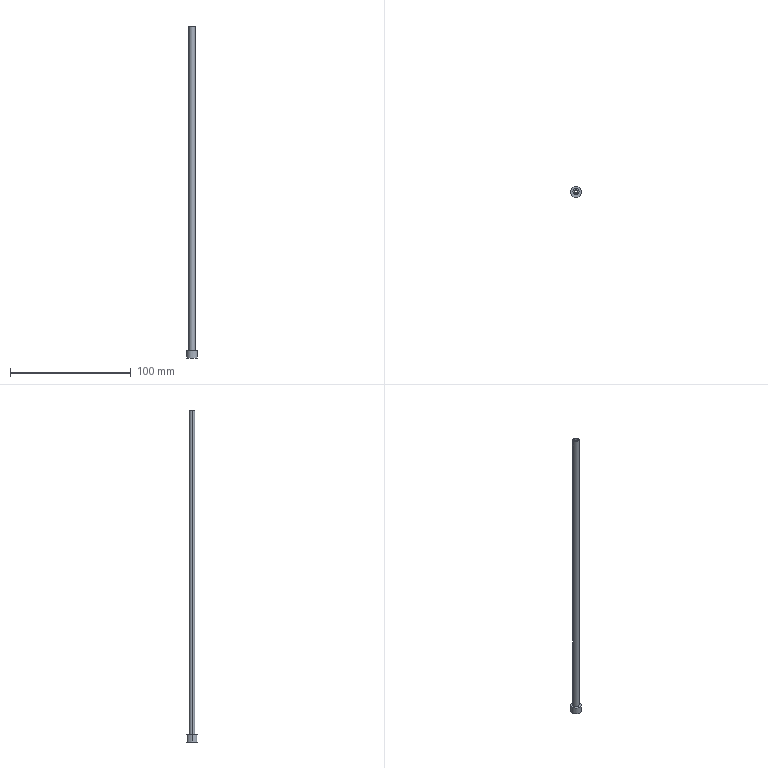Part | Creo | 1 solid | 12 faces | box 9 x 9 x 275.272 mm | volume 3782 mm3 | cylinder 8 | plane 4 | commonest cylinder face diameters 2.8 x2 3 x2 5 x2 9 x2
STEP:
#1=CARTESIAN_POINT('',(52.238,-56.28,-296.));
#2=VERTEX_POINT('',#1);
#3=CARTESIAN_POINT('',(43.238,-56.28,-296.));
#4=VERTEX_POINT('',#3);
#5=CARTESIAN_POINT('',(47.738,-56.28,-296.));
#6=DIRECTION('',(0.,0.,-1.));
#7=DIRECTION('',(1.,0.,0.));
#8=AXIS2_PLACEMENT_3D('',#5,#6,#7);
#9=CIRCLE('',#8,4.5);
#10=EDGE_CURVE('',#2,#4,#9,.T.);
#11=ORIENTED_EDGE('',*,*,#10,.F.);
#12=CARTESIAN_POINT('',(47.738,-56.28,-296.));
#13=DIRECTION('',(0.,0.,-1.));
#14=DIRECTION('',(-1.,0.,0.));
#15=AXIS2_PLACEMENT_3D('',#12,#13,#14);
#16=CIRCLE('',#15,4.5);
#17=EDGE_CURVE('',#4,#2,#16,.T.);
#18=ORIENTED_EDGE('',*,*,#17,.F.);
#19=EDGE_LOOP('',(#11,#18));
#20=FACE_OUTER_BOUND('',#19,.F.);
#21=CARTESIAN_POINT('',(49.238,-56.28,-296.));
#22=VERTEX_POINT('',#21);
#23=CARTESIAN_POINT('',(46.238,-56.28,-296.));
#24=VERTEX_POINT('',#23);
#25=CARTESIAN_POINT('',(47.738,-56.28,-296.));
#26=DIRECTION('',(0.,0.,1.));
#27=DIRECTION('',(1.,0.,0.));
#28=AXIS2_PLACEMENT_3D('',#25,#26,#27);
#29=CIRCLE('',#28,1.5);
#30=EDGE_CURVE('',#22,#24,#29,.T.);
#31=ORIENTED_EDGE('',*,*,#30,.F.);
#32=CARTESIAN_POINT('',(47.738,-56.28,-296.));
#33=DIRECTION('',(0.,0.,1.));
#34=DIRECTION('',(-1.,0.,0.));
#35=AXIS2_PLACEMENT_3D('',#32,#33,#34);
#36=CIRCLE('',#35,1.5);
#37=EDGE_CURVE('',#24,#22,#36,.T.);
#38=ORIENTED_EDGE('',*,*,#37,.F.);
#39=EDGE_LOOP('',(#31,#38));
#40=FACE_BOUND('',#39,.F.);
#41=CARTESIAN_POINT('',(10.,-0.004699,-296.));
#42=DIRECTION('',(0.,0.,1.));
#43=DIRECTION('',(0.,1.,0.));
#44=AXIS2_PLACEMENT_3D('',#41,#42,#43);
#45=PLANE('',#44);
#46=ADVANCED_FACE('',(#20,#40),#45,.F.);
#47=CARTESIAN_POINT('',(43.238,-56.28,-290.));
#48=VERTEX_POINT('',#47);
#49=CARTESIAN_POINT('',(52.238,-56.28,-290.));
#50=VERTEX_POINT('',#49);
#51=CARTESIAN_POINT('',(47.738,-56.28,-290.));
#52=DIRECTION('',(0.,0.,1.));
#53=DIRECTION('',(-1.,0.,0.));
#54=AXIS2_PLACEMENT_3D('',#51,#52,#53);
#55=CIRCLE('',#54,4.5);
#56=EDGE_CURVE('',#48,#50,#55,.T.);
#57=ORIENTED_EDGE('',*,*,#56,.T.);
#58=CARTESIAN_POINT('',(52.238,-56.28,-296.));
#59=DIRECTION('',(0.,0.,1.));
#60=VECTOR('',#59,6.);
#61=LINE('',#58,#60);
#62=EDGE_CURVE('',#2,#50,#61,.T.);
#63=ORIENTED_EDGE('',*,*,#62,.F.);
#64=ORIENTED_EDGE('',*,*,#10,.T.);
#65=CARTESIAN_POINT('',(43.238,-56.28,-296.));
#66=DIRECTION('',(0.,0.,1.));
#67=VECTOR('',#66,6.);
#68=LINE('',#65,#67);
#69=EDGE_CURVE('',#4,#48,#68,.T.);
#70=ORIENTED_EDGE('',*,*,#69,.T.);
#71=EDGE_LOOP('',(#57,#63,#64,#70));
#72=FACE_OUTER_BOUND('',#71,.F.);
#73=CARTESIAN_POINT('',(47.738,-56.28,-296.));
#74=DIRECTION('',(0.,0.,1.));
#75=DIRECTION('',(-1.,0.,0.));
#76=AXIS2_PLACEMENT_3D('',#73,#74,#75);
#77=CYLINDRICAL_SURFACE('',#76,4.5);
#78=ADVANCED_FACE('',(#72),#77,.T.);
#79=CARTESIAN_POINT('',(47.738,-56.28,-290.));
#80=DIRECTION('',(0.,0.,1.));
#81=DIRECTION('',(1.,0.,0.));
#82=AXIS2_PLACEMENT_3D('',#79,#80,#81);
#83=CIRCLE('',#82,4.5);
#84=EDGE_CURVE('',#50,#48,#83,.T.);
#85=ORIENTED_EDGE('',*,*,#84,.F.);
#86=ORIENTED_EDGE('',*,*,#56,.F.);
#87=EDGE_LOOP('',(#85,#86));
#88=FACE_OUTER_BOUND('',#87,.F.);
#89=CARTESIAN_POINT('',(50.238,-56.28,-290.));
#90=VERTEX_POINT('',#89);
#91=CARTESIAN_POINT('',(45.238,-56.28,-290.));
#92=VERTEX_POINT('',#91);
#93=CARTESIAN_POINT('',(47.738,-56.28,-290.));
#94=DIRECTION('',(0.,0.,-1.));
#95=DIRECTION('',(1.,0.,0.));
#96=AXIS2_PLACEMENT_3D('',#93,#94,#95);
#97=CIRCLE('',#96,2.5);
#98=EDGE_CURVE('',#90,#92,#97,.T.);
#99=ORIENTED_EDGE('',*,*,#98,.F.);
#100=CARTESIAN_POINT('',(47.738,-56.28,-290.));
#101=DIRECTION('',(0.,0.,-1.));
#102=DIRECTION('',(-1.,0.,0.));
#103=AXIS2_PLACEMENT_3D('',#100,#101,#102);
#104=CIRCLE('',#103,2.5);
#105=EDGE_CURVE('',#92,#90,#104,.T.);
#106=ORIENTED_EDGE('',*,*,#105,.F.);
#107=EDGE_LOOP('',(#99,#106));
#108=FACE_BOUND('',#107,.F.);
#109=CARTESIAN_POINT('',(47.738,-56.28,-290.));
#110=DIRECTION('',(0.,0.,1.));
#111=DIRECTION('',(-1.,0.,0.));
#112=AXIS2_PLACEMENT_3D('',#109,#110,#111);
#113=PLANE('',#112);
#114=ADVANCED_FACE('',(#88,#108),#113,.T.);
#115=ORIENTED_EDGE('',*,*,#98,.T.);
#116=CARTESIAN_POINT('',(45.238,-56.28,-20.728));
#117=VERTEX_POINT('',#116);
#118=CARTESIAN_POINT('',(45.238,-56.28,-290.));
#119=DIRECTION('',(0.,0.,1.));
#120=VECTOR('',#119,269.272);
#121=LINE('',#118,#120);
#122=EDGE_CURVE('',#92,#117,#121,.T.);
#123=ORIENTED_EDGE('',*,*,#122,.T.);
#124=CARTESIAN_POINT('',(50.238,-56.28,-20.728));
#125=VERTEX_POINT('',#124);
#126=CARTESIAN_POINT('',(47.738,-56.28,-20.728));
#127=DIRECTION('',(0.,0.,1.));
#128=DIRECTION('',(-1.,0.,0.));
#129=AXIS2_PLACEMENT_3D('',#126,#127,#128);
#130=CIRCLE('',#129,2.5);
#131=EDGE_CURVE('',#117,#125,#130,.T.);
#132=ORIENTED_EDGE('',*,*,#131,.T.);
#133=CARTESIAN_POINT('',(50.238,-56.28,-290.));
#134=DIRECTION('',(0.,0.,1.));
#135=VECTOR('',#134,269.272);
#136=LINE('',#133,#135);
#137=EDGE_CURVE('',#90,#125,#136,.T.);
#138=ORIENTED_EDGE('',*,*,#137,.F.);
#139=EDGE_LOOP('',(#115,#123,#132,#138));
#140=FACE_OUTER_BOUND('',#139,.F.);
#141=CARTESIAN_POINT('',(47.738,-56.28,-335.923));
#142=DIRECTION('',(0.,0.,1.));
#143=DIRECTION('',(1.,0.,0.));
#144=AXIS2_PLACEMENT_3D('',#141,#142,#143);
#145=CYLINDRICAL_SURFACE('',#144,2.5);
#146=ADVANCED_FACE('',(#140),#145,.T.);
#147=ORIENTED_EDGE('',*,*,#105,.T.);
#148=ORIENTED_EDGE('',*,*,#137,.T.);
#149=CARTESIAN_POINT('',(47.738,-56.28,-20.728));
#150=DIRECTION('',(0.,0.,1.));
#151=DIRECTION('',(1.,0.,0.));
#152=AXIS2_PLACEMENT_3D('',#149,#150,#151);
#153=CIRCLE('',#152,2.5);
#154=EDGE_CURVE('',#125,#117,#153,.T.);
#155=ORIENTED_EDGE('',*,*,#154,.T.);
#156=ORIENTED_EDGE('',*,*,#122,.F.);
#157=EDGE_LOOP('',(#147,#148,#155,#156));
#158=FACE_OUTER_BOUND('',#157,.F.);
#159=CARTESIAN_POINT('',(47.738,-56.28,-335.923));
#160=DIRECTION('',(0.,0.,1.));
#161=DIRECTION('',(1.,0.,0.));
#162=AXIS2_PLACEMENT_3D('',#159,#160,#161);
#163=CYLINDRICAL_SURFACE('',#162,2.5);
#164=ADVANCED_FACE('',(#158),#163,.T.);
#165=ORIENTED_EDGE('',*,*,#154,.F.);
#166=ORIENTED_EDGE('',*,*,#131,.F.);
#167=EDGE_LOOP('',(#165,#166));
#168=FACE_OUTER_BOUND('',#167,.F.);
#169=CARTESIAN_POINT('',(49.138,-56.28,-20.728));
#170=VERTEX_POINT('',#169);
#171=CARTESIAN_POINT('',(46.338,-56.28,-20.728));
#172=VERTEX_POINT('',#171);
#173=CARTESIAN_POINT('',(47.738,-56.28,-20.728));
#174=DIRECTION('',(0.,0.,-1.));
#175=DIRECTION('',(1.,0.,0.));
#176=AXIS2_PLACEMENT_3D('',#173,#174,#175);
#177=CIRCLE('',#176,1.4);
#178=EDGE_CURVE('',#170,#172,#177,.T.);
#179=ORIENTED_EDGE('',*,*,#178,.F.);
#180=CARTESIAN_POINT('',(47.738,-56.28,-20.728));
#181=DIRECTION('',(0.,0.,-1.));
#182=DIRECTION('',(-1.,0.,0.));
#183=AXIS2_PLACEMENT_3D('',#180,#181,#182);
#184=CIRCLE('',#183,1.4);
#185=EDGE_CURVE('',#172,#170,#184,.T.);
#186=ORIENTED_EDGE('',*,*,#185,.F.);
#187=EDGE_LOOP('',(#179,#186));
#188=FACE_BOUND('',#187,.F.);
#189=CARTESIAN_POINT('',(47.738,-56.28,-20.728));
#190=DIRECTION('',(0.,0.,1.));
#191=DIRECTION('',(1.,0.,0.));
#192=AXIS2_PLACEMENT_3D('',#189,#190,#191);
#193=PLANE('',#192);
#194=ADVANCED_FACE('',(#168,#188),#193,.T.);
#195=CARTESIAN_POINT('',(46.338,-56.28,-85.923));
#196=VERTEX_POINT('',#195);
#197=CARTESIAN_POINT('',(49.138,-56.28,-85.923));
#198=VERTEX_POINT('',#197);
#199=CARTESIAN_POINT('',(47.738,-56.28,-85.923));
#200=DIRECTION('',(0.,0.,1.));
#201=DIRECTION('',(-1.,0.,0.));
#202=AXIS2_PLACEMENT_3D('',#199,#200,#201);
#203=CIRCLE('',#202,1.4);
#204=EDGE_CURVE('',#196,#198,#203,.T.);
#205=ORIENTED_EDGE('',*,*,#204,.T.);
#206=CARTESIAN_POINT('',(49.138,-56.28,-85.923));
#207=DIRECTION('',(0.,0.,1.));
#208=VECTOR('',#207,65.195);
#209=LINE('',#206,#208);
#210=EDGE_CURVE('',#198,#170,#209,.T.);
#211=ORIENTED_EDGE('',*,*,#210,.T.);
#212=ORIENTED_EDGE('',*,*,#178,.T.);
#213=CARTESIAN_POINT('',(46.338,-56.28,-85.923));
#214=DIRECTION('',(0.,0.,1.));
#215=VECTOR('',#214,65.195);
#216=LINE('',#213,#215);
#217=EDGE_CURVE('',#196,#172,#216,.T.);
#218=ORIENTED_EDGE('',*,*,#217,.F.);
#219=EDGE_LOOP('',(#205,#211,#212,#218));
#220=FACE_OUTER_BOUND('',#219,.F.);
#221=CARTESIAN_POINT('',(47.738,-56.28,-335.923));
#222=DIRECTION('',(0.,0.,1.));
#223=DIRECTION('',(1.,0.,0.));
#224=AXIS2_PLACEMENT_3D('',#221,#222,#223);
#225=CYLINDRICAL_SURFACE('',#224,1.4);
#226=ADVANCED_FACE('',(#220),#225,.F.);
#227=CARTESIAN_POINT('',(49.238,-56.28,-85.923));
#228=VERTEX_POINT('',#227);
#229=CARTESIAN_POINT('',(46.238,-56.28,-85.923));
#230=VERTEX_POINT('',#229);
#231=CARTESIAN_POINT('',(47.738,-56.28,-85.923));
#232=DIRECTION('',(0.,0.,-1.));
#233=DIRECTION('',(1.,0.,0.));
#234=AXIS2_PLACEMENT_3D('',#231,#232,#233);
#235=CIRCLE('',#234,1.5);
#236=EDGE_CURVE('',#228,#230,#235,.T.);
#237=ORIENTED_EDGE('',*,*,#236,.F.);
#238=CARTESIAN_POINT('',(47.738,-56.28,-85.923));
#239=DIRECTION('',(0.,0.,-1.));
#240=DIRECTION('',(-1.,0.,0.));
#241=AXIS2_PLACEMENT_3D('',#238,#239,#240);
#242=CIRCLE('',#241,1.5);
#243=EDGE_CURVE('',#230,#228,#242,.T.);
#244=ORIENTED_EDGE('',*,*,#243,.F.);
#245=EDGE_LOOP('',(#237,#244));
#246=FACE_OUTER_BOUND('',#245,.F.);
#247=CARTESIAN_POINT('',(47.738,-56.28,-85.923));
#248=DIRECTION('',(0.,0.,1.));
#249=DIRECTION('',(1.,0.,0.));
#250=AXIS2_PLACEMENT_3D('',#247,#248,#249);
#251=CIRCLE('',#250,1.4);
#252=EDGE_CURVE('',#198,#196,#251,.T.);
#253=ORIENTED_EDGE('',*,*,#252,.F.);
#254=ORIENTED_EDGE('',*,*,#204,.F.);
#255=EDGE_LOOP('',(#253,#254));
#256=FACE_BOUND('',#255,.F.);
#257=CARTESIAN_POINT('',(47.738,-56.28,-85.923));
#258=DIRECTION('',(0.,0.,1.));
#259=DIRECTION('',(1.,0.,0.));
#260=AXIS2_PLACEMENT_3D('',#257,#258,#259);
#261=PLANE('',#260);
#262=ADVANCED_FACE('',(#246,#256),#261,.F.);
#263=ORIENTED_EDGE('',*,*,#37,.T.);
#264=CARTESIAN_POINT('',(49.238,-56.28,-296.));
#265=DIRECTION('',(0.,0.,1.));
#266=VECTOR('',#265,210.077);
#267=LINE('',#264,#266);
#268=EDGE_CURVE('',#22,#228,#267,.T.);
#269=ORIENTED_EDGE('',*,*,#268,.T.);
#270=ORIENTED_EDGE('',*,*,#236,.T.);
#271=CARTESIAN_POINT('',(46.238,-56.28,-296.));
#272=DIRECTION('',(0.,0.,1.));
#273=VECTOR('',#272,210.077);
#274=LINE('',#271,#273);
#275=EDGE_CURVE('',#24,#230,#274,.T.);
#276=ORIENTED_EDGE('',*,*,#275,.F.);
#277=EDGE_LOOP('',(#263,#269,#270,#276));
#278=FACE_OUTER_BOUND('',#277,.F.);
#279=CARTESIAN_POINT('',(47.738,-56.28,-335.923));
#280=DIRECTION('',(0.,0.,1.));
#281=DIRECTION('',(1.,0.,0.));
#282=AXIS2_PLACEMENT_3D('',#279,#280,#281);
#283=CYLINDRICAL_SURFACE('',#282,1.5);
#284=ADVANCED_FACE('',(#278),#283,.F.);
#285=ORIENTED_EDGE('',*,*,#30,.T.);
#286=ORIENTED_EDGE('',*,*,#275,.T.);
#287=ORIENTED_EDGE('',*,*,#243,.T.);
#288=ORIENTED_EDGE('',*,*,#268,.F.);
#289=EDGE_LOOP('',(#285,#286,#287,#288));
#290=FACE_OUTER_BOUND('',#289,.F.);
#291=CARTESIAN_POINT('',(47.738,-56.28,-335.923));
#292=DIRECTION('',(0.,0.,1.));
#293=DIRECTION('',(1.,0.,0.));
#294=AXIS2_PLACEMENT_3D('',#291,#292,#293);
#295=CYLINDRICAL_SURFACE('',#294,1.5);
#296=ADVANCED_FACE('',(#290),#295,.F.);
#297=ORIENTED_EDGE('',*,*,#252,.T.);
#298=ORIENTED_EDGE('',*,*,#217,.T.);
#299=ORIENTED_EDGE('',*,*,#185,.T.);
#300=ORIENTED_EDGE('',*,*,#210,.F.);
#301=EDGE_LOOP('',(#297,#298,#299,#300));
#302=FACE_OUTER_BOUND('',#301,.F.);
#303=CARTESIAN_POINT('',(47.738,-56.28,-335.923));
#304=DIRECTION('',(0.,0.,1.));
#305=DIRECTION('',(1.,0.,0.));
#306=AXIS2_PLACEMENT_3D('',#303,#304,#305);
#307=CYLINDRICAL_SURFACE('',#306,1.4);
#308=ADVANCED_FACE('',(#302),#307,.F.);
#309=ORIENTED_EDGE('',*,*,#84,.T.);
#310=ORIENTED_EDGE('',*,*,#69,.F.);
#311=ORIENTED_EDGE('',*,*,#17,.T.);
#312=ORIENTED_EDGE('',*,*,#62,.T.);
#313=EDGE_LOOP('',(#309,#310,#311,#312));
#314=FACE_OUTER_BOUND('',#313,.F.);
#315=CARTESIAN_POINT('',(47.738,-56.28,-296.));
#316=DIRECTION('',(0.,0.,1.));
#317=DIRECTION('',(-1.,0.,0.));
#318=AXIS2_PLACEMENT_3D('',#315,#316,#317);
#319=CYLINDRICAL_SURFACE('',#318,4.5);
#320=ADVANCED_FACE('',(#314),#319,.T.);
#321=CLOSED_SHELL('',(#46,#78,#114,#146,#164,#194,#226,#262,#284,#296,#308,#320));
#322=MANIFOLD_SOLID_BREP('',#321);
#323=(LENGTH_UNIT()NAMED_UNIT(*)SI_UNIT(.MILLI.,.METRE.));
#324=UNCERTAINTY_MEASURE_WITH_UNIT(LENGTH_MEASURE(0.02756),#323,'','');
#325=(NAMED_UNIT(*)PLANE_ANGLE_UNIT()SI_UNIT($,.RADIAN.));
#326=PLANE_ANGLE_MEASURE_WITH_UNIT(PLANE_ANGLE_MEASURE(0.01745),#325);
#327=(CONVERSION_BASED_UNIT('DEGREE',#326)NAMED_UNIT(*)PLANE_ANGLE_UNIT());
#328=(NAMED_UNIT(*)SI_UNIT($,.STERADIAN.)SOLID_ANGLE_UNIT());
#329=(GEOMETRIC_REPRESENTATION_CONTEXT(3)GLOBAL_UNCERTAINTY_ASSIGNED_CONTEXT((#324))GLOBAL_UNIT_ASSIGNED_CONTEXT((#323,#327,#328))REPRESENTATION_CONTEXT('',''));
#330=ADVANCED_BREP_SHAPE_REPRESENTATION('',(#322),#329);